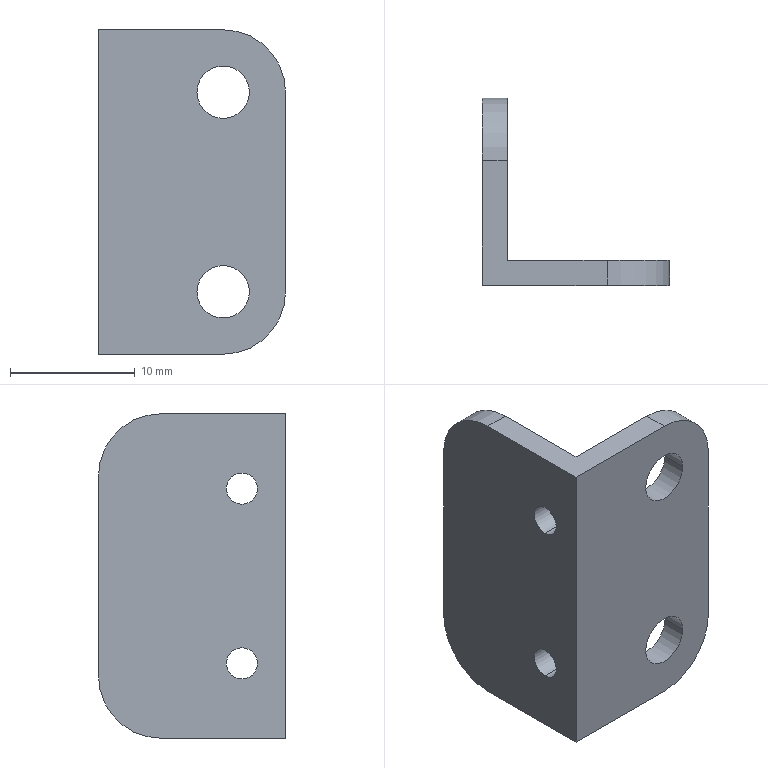Part | STEP file | Sensor mount plate | 1 solid | 20 faces | box 15 x 15 x 26 mm | volume 1338 mm3 | cylinder 12 | plane 8 | commonest cylinder face diameters 2.5 x4 4.2 x4 10 x4